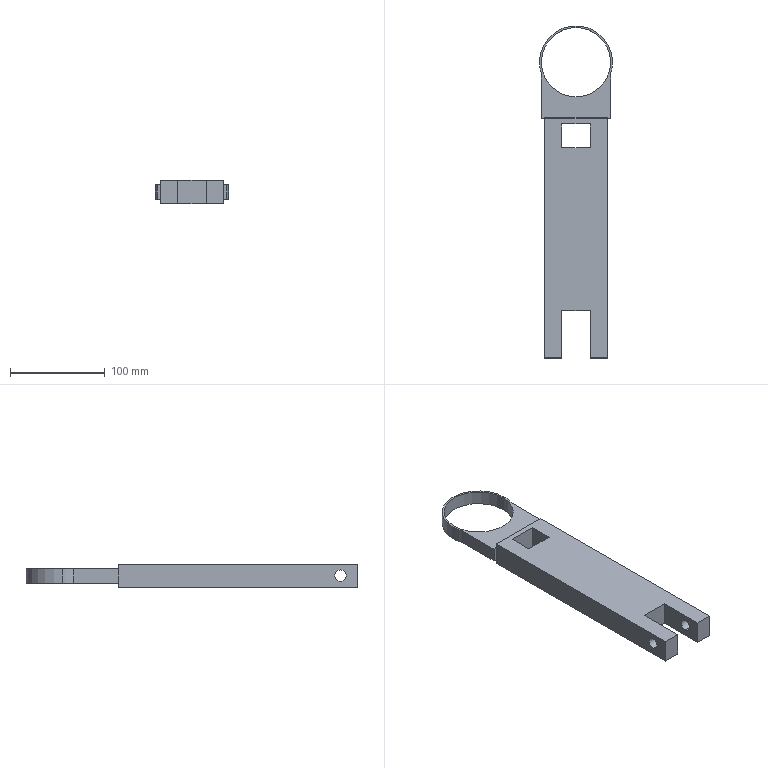Part | SolidWorks | features ICE 3, 3DProfileFeature 1, BossThin 1, Extrusion 1, Fillet 1, HoleWzd 1, MirrorPattern 1 | 1 solid | 32 faces | box 77 x 350 x 25 mm | volume 393296 mm3 | plane 21 | cylinder 11 | commonest cylinder face diameters 12 x4 77 x3 2 x2 73 x2
STEP:
#1=CARTESIAN_POINT('',(-38.5,161.5,-7.5));
#2=VERTEX_POINT('',#1);
#3=CARTESIAN_POINT('',(38.5,161.5,-7.5));
#4=VERTEX_POINT('',#3);
#5=CARTESIAN_POINT('',(0.,161.5,-7.5));
#6=DIRECTION('',(0.,0.,-1.));
#7=DIRECTION('',(-1.,0.,0.));
#8=AXIS2_PLACEMENT_3D('',#5,#6,#7);
#9=CIRCLE('',#8,38.5);
#10=EDGE_CURVE('',#2,#4,#9,.T.);
#11=ORIENTED_EDGE('',*,*,#10,.F.);
#12=CARTESIAN_POINT('',(-38.5,161.5,7.5));
#13=VERTEX_POINT('',#12);
#14=CARTESIAN_POINT('',(-38.5,161.5,-7.5));
#15=DIRECTION('',(0.,0.,1.));
#16=VECTOR('',#15,1000.);
#17=LINE('',#14,#16);
#18=EDGE_CURVE('',#2,#13,#17,.T.);
#19=ORIENTED_EDGE('',*,*,#18,.T.);
#20=CARTESIAN_POINT('',(38.5,161.5,7.5));
#21=VERTEX_POINT('',#20);
#22=CARTESIAN_POINT('',(0.,161.5,7.5));
#23=DIRECTION('',(0.,0.,-1.));
#24=DIRECTION('',(-1.,0.,0.));
#25=AXIS2_PLACEMENT_3D('',#22,#23,#24);
#26=CIRCLE('',#25,38.5);
#27=EDGE_CURVE('',#13,#21,#26,.T.);
#28=ORIENTED_EDGE('',*,*,#27,.T.);
#29=CARTESIAN_POINT('',(38.5,161.5,-7.5));
#30=DIRECTION('',(0.,0.,1.));
#31=VECTOR('',#30,1000.);
#32=LINE('',#29,#31);
#33=EDGE_CURVE('',#4,#21,#32,.T.);
#34=ORIENTED_EDGE('',*,*,#33,.F.);
#35=EDGE_LOOP('',(#11,#19,#28,#34));
#36=FACE_OUTER_BOUND('',#35,.T.);
#37=CARTESIAN_POINT('',(0.,161.5,-7.5));
#38=DIRECTION('',(0.,0.,1.));
#39=DIRECTION('',(1.,0.,0.));
#40=AXIS2_PLACEMENT_3D('',#37,#38,#39);
#41=CYLINDRICAL_SURFACE('',#40,38.5);
#42=ADVANCED_FACE('',(#36),#41,.T.);
#43=CARTESIAN_POINT('',(36.5,149.253,-7.5));
#44=VERTEX_POINT('',#43);
#45=CARTESIAN_POINT('',(0.,161.5,-7.5));
#46=DIRECTION('',(0.,0.,-1.));
#47=DIRECTION('',(-1.,0.,0.));
#48=AXIS2_PLACEMENT_3D('',#45,#46,#47);
#49=CIRCLE('',#48,38.5);
#50=EDGE_CURVE('',#4,#44,#49,.T.);
#51=ORIENTED_EDGE('',*,*,#50,.F.);
#52=ORIENTED_EDGE('',*,*,#33,.T.);
#53=CARTESIAN_POINT('',(36.5,149.253,7.5));
#54=VERTEX_POINT('',#53);
#55=CARTESIAN_POINT('',(0.,161.5,7.5));
#56=DIRECTION('',(0.,0.,-1.));
#57=DIRECTION('',(-1.,0.,0.));
#58=AXIS2_PLACEMENT_3D('',#55,#56,#57);
#59=CIRCLE('',#58,38.5);
#60=EDGE_CURVE('',#21,#54,#59,.T.);
#61=ORIENTED_EDGE('',*,*,#60,.T.);
#62=CARTESIAN_POINT('',(36.5,149.253,-7.5));
#63=DIRECTION('',(0.,0.,-1.));
#64=VECTOR('',#63,1000.);
#65=LINE('',#62,#64);
#66=EDGE_CURVE('',#54,#44,#65,.T.);
#67=ORIENTED_EDGE('',*,*,#66,.T.);
#68=EDGE_LOOP('',(#51,#52,#61,#67));
#69=FACE_OUTER_BOUND('',#68,.T.);
#70=CARTESIAN_POINT('',(0.,161.5,-7.5));
#71=DIRECTION('',(0.,0.,1.));
#72=DIRECTION('',(1.,0.,0.));
#73=AXIS2_PLACEMENT_3D('',#70,#71,#72);
#74=CYLINDRICAL_SURFACE('',#73,38.5);
#75=ADVANCED_FACE('',(#69),#74,.T.);
#76=CARTESIAN_POINT('',(36.5,161.5,-7.5));
#77=VERTEX_POINT('',#76);
#78=CARTESIAN_POINT('',(-36.5,161.5,-7.5));
#79=VERTEX_POINT('',#78);
#80=CARTESIAN_POINT('',(0.,161.5,-7.5));
#81=DIRECTION('',(0.,0.,-1.));
#82=DIRECTION('',(-1.,0.,0.));
#83=AXIS2_PLACEMENT_3D('',#80,#81,#82);
#84=CIRCLE('',#83,36.5);
#85=EDGE_CURVE('',#77,#79,#84,.T.);
#86=ORIENTED_EDGE('',*,*,#85,.T.);
#87=CARTESIAN_POINT('',(-36.5,161.5,7.5));
#88=VERTEX_POINT('',#87);
#89=CARTESIAN_POINT('',(-36.5,161.5,-7.5));
#90=DIRECTION('',(0.,0.,1.));
#91=VECTOR('',#90,1000.);
#92=LINE('',#89,#91);
#93=EDGE_CURVE('',#79,#88,#92,.T.);
#94=ORIENTED_EDGE('',*,*,#93,.T.);
#95=CARTESIAN_POINT('',(36.5,161.5,7.5));
#96=VERTEX_POINT('',#95);
#97=CARTESIAN_POINT('',(0.,161.5,7.5));
#98=DIRECTION('',(0.,0.,-1.));
#99=DIRECTION('',(-1.,0.,0.));
#100=AXIS2_PLACEMENT_3D('',#97,#98,#99);
#101=CIRCLE('',#100,36.5);
#102=EDGE_CURVE('',#96,#88,#101,.T.);
#103=ORIENTED_EDGE('',*,*,#102,.F.);
#104=CARTESIAN_POINT('',(36.5,161.5,-7.5));
#105=DIRECTION('',(0.,0.,1.));
#106=VECTOR('',#105,1000.);
#107=LINE('',#104,#106);
#108=EDGE_CURVE('',#77,#96,#107,.T.);
#109=ORIENTED_EDGE('',*,*,#108,.F.);
#110=EDGE_LOOP('',(#86,#94,#103,#109));
#111=FACE_OUTER_BOUND('',#110,.T.);
#112=CARTESIAN_POINT('',(0.,161.5,-7.5));
#113=DIRECTION('',(0.,0.,1.));
#114=DIRECTION('',(1.,0.,0.));
#115=AXIS2_PLACEMENT_3D('',#112,#113,#114);
#116=CYLINDRICAL_SURFACE('',#115,36.5);
#117=ADVANCED_FACE('',(#111),#116,.F.);
#118=CARTESIAN_POINT('',(-15.,-131.5,-5.548));
#119=VERTEX_POINT('',#118);
#120=CARTESIAN_POINT('',(-15.,-131.5,6.452));
#121=VERTEX_POINT('',#120);
#122=CARTESIAN_POINT('',(-15.,-131.5,0.4516));
#123=DIRECTION('',(-1.,0.,0.));
#124=DIRECTION('',(0.,0.,1.));
#125=AXIS2_PLACEMENT_3D('',#122,#123,#124);
#126=CIRCLE('',#125,6.);
#127=EDGE_CURVE('',#119,#121,#126,.T.);
#128=ORIENTED_EDGE('',*,*,#127,.F.);
#129=CARTESIAN_POINT('',(-33.,-131.5,-5.548));
#130=VERTEX_POINT('',#129);
#131=CARTESIAN_POINT('',(-33.,-131.5,-5.548));
#132=DIRECTION('',(-1.,0.,0.));
#133=VECTOR('',#132,1000.);
#134=LINE('',#131,#133);
#135=EDGE_CURVE('',#119,#130,#134,.T.);
#136=ORIENTED_EDGE('',*,*,#135,.T.);
#137=CARTESIAN_POINT('',(-33.,-131.5,6.452));
#138=VERTEX_POINT('',#137);
#139=CARTESIAN_POINT('',(-33.,-131.5,0.4516));
#140=DIRECTION('',(-1.,0.,0.));
#141=DIRECTION('',(0.,0.,1.));
#142=AXIS2_PLACEMENT_3D('',#139,#140,#141);
#143=CIRCLE('',#142,6.);
#144=EDGE_CURVE('',#130,#138,#143,.T.);
#145=ORIENTED_EDGE('',*,*,#144,.T.);
#146=CARTESIAN_POINT('',(-33.,-131.5,6.452));
#147=DIRECTION('',(-1.,0.,0.));
#148=VECTOR('',#147,1000.);
#149=LINE('',#146,#148);
#150=EDGE_CURVE('',#121,#138,#149,.T.);
#151=ORIENTED_EDGE('',*,*,#150,.F.);
#152=EDGE_LOOP('',(#128,#136,#145,#151));
#153=FACE_OUTER_BOUND('',#152,.T.);
#154=CARTESIAN_POINT('',(-33.,-131.5,0.4516));
#155=DIRECTION('',(-1.,0.,0.));
#156=DIRECTION('',(0.,0.,1.));
#157=AXIS2_PLACEMENT_3D('',#154,#155,#156);
#158=CYLINDRICAL_SURFACE('',#157,6.);
#159=ADVANCED_FACE('',(#153),#158,.F.);
#160=CARTESIAN_POINT('',(15.,-131.5,6.452));
#161=VERTEX_POINT('',#160);
#162=CARTESIAN_POINT('',(15.,-131.5,-5.548));
#163=VERTEX_POINT('',#162);
#164=CARTESIAN_POINT('',(15.,-131.5,0.4516));
#165=DIRECTION('',(1.,0.,0.));
#166=DIRECTION('',(0.,1.,0.));
#167=AXIS2_PLACEMENT_3D('',#164,#165,#166);
#168=CIRCLE('',#167,6.);
#169=EDGE_CURVE('',#161,#163,#168,.T.);
#170=ORIENTED_EDGE('',*,*,#169,.F.);
#171=CARTESIAN_POINT('',(33.,-131.5,6.452));
#172=VERTEX_POINT('',#171);
#173=CARTESIAN_POINT('',(33.,-131.5,6.452));
#174=DIRECTION('',(1.,0.,0.));
#175=VECTOR('',#174,1000.);
#176=LINE('',#173,#175);
#177=EDGE_CURVE('',#161,#172,#176,.T.);
#178=ORIENTED_EDGE('',*,*,#177,.T.);
#179=CARTESIAN_POINT('',(33.,-131.5,-5.548));
#180=VERTEX_POINT('',#179);
#181=CARTESIAN_POINT('',(33.,-131.5,0.4516));
#182=DIRECTION('',(1.,0.,0.));
#183=DIRECTION('',(0.,0.,-1.));
#184=AXIS2_PLACEMENT_3D('',#181,#182,#183);
#185=CIRCLE('',#184,6.);
#186=EDGE_CURVE('',#172,#180,#185,.T.);
#187=ORIENTED_EDGE('',*,*,#186,.T.);
#188=CARTESIAN_POINT('',(33.,-131.5,-5.548));
#189=DIRECTION('',(1.,0.,0.));
#190=VECTOR('',#189,1000.);
#191=LINE('',#188,#190);
#192=EDGE_CURVE('',#163,#180,#191,.T.);
#193=ORIENTED_EDGE('',*,*,#192,.F.);
#194=EDGE_LOOP('',(#170,#178,#187,#193));
#195=FACE_OUTER_BOUND('',#194,.T.);
#196=CARTESIAN_POINT('',(33.,-131.5,0.4516));
#197=DIRECTION('',(1.,0.,0.));
#198=DIRECTION('',(0.,0.,-1.));
#199=AXIS2_PLACEMENT_3D('',#196,#197,#198);
#200=CYLINDRICAL_SURFACE('',#199,6.);
#201=ADVANCED_FACE('',(#195),#200,.F.);
#202=CARTESIAN_POINT('',(-36.5,149.253,7.5));
#203=VERTEX_POINT('',#202);
#204=CARTESIAN_POINT('',(-36.5,102.,7.5));
#205=VERTEX_POINT('',#204);
#206=CARTESIAN_POINT('',(-36.5,0.,7.5));
#207=DIRECTION('',(0.,-1.,0.));
#208=VECTOR('',#207,1000.);
#209=LINE('',#206,#208);
#210=EDGE_CURVE('',#203,#205,#209,.T.);
#211=ORIENTED_EDGE('',*,*,#210,.F.);
#212=CARTESIAN_POINT('',(-36.5,149.253,-7.5));
#213=VERTEX_POINT('',#212);
#214=CARTESIAN_POINT('',(-36.5,149.253,-7.5));
#215=DIRECTION('',(0.,0.,-1.));
#216=VECTOR('',#215,1000.);
#217=LINE('',#214,#216);
#218=EDGE_CURVE('',#203,#213,#217,.T.);
#219=ORIENTED_EDGE('',*,*,#218,.T.);
#220=CARTESIAN_POINT('',(-36.5,102.,-7.5));
#221=VERTEX_POINT('',#220);
#222=CARTESIAN_POINT('',(-36.5,0.,-7.5));
#223=DIRECTION('',(0.,-1.,0.));
#224=VECTOR('',#223,1000.);
#225=LINE('',#222,#224);
#226=EDGE_CURVE('',#213,#221,#225,.T.);
#227=ORIENTED_EDGE('',*,*,#226,.T.);
#228=CARTESIAN_POINT('',(-36.5,102.,-7.5));
#229=DIRECTION('',(0.,0.,1.));
#230=VECTOR('',#229,1000.);
#231=LINE('',#228,#230);
#232=EDGE_CURVE('',#221,#205,#231,.T.);
#233=ORIENTED_EDGE('',*,*,#232,.T.);
#234=EDGE_LOOP('',(#211,#219,#227,#233));
#235=FACE_OUTER_BOUND('',#234,.T.);
#236=CARTESIAN_POINT('',(-36.5,0.,-7.5));
#237=DIRECTION('',(-1.,0.,0.));
#238=DIRECTION('',(0.,-1.,0.));
#239=AXIS2_PLACEMENT_3D('',#236,#237,#238);
#240=PLANE('',#239);
#241=ADVANCED_FACE('',(#235),#240,.T.);
#242=ORIENTED_EDGE('',*,*,#66,.F.);
#243=CARTESIAN_POINT('',(36.5,102.,7.5));
#244=VERTEX_POINT('',#243);
#245=CARTESIAN_POINT('',(36.5,0.,7.5));
#246=DIRECTION('',(0.,-1.,0.));
#247=VECTOR('',#246,1000.);
#248=LINE('',#245,#247);
#249=EDGE_CURVE('',#54,#244,#248,.T.);
#250=ORIENTED_EDGE('',*,*,#249,.T.);
#251=CARTESIAN_POINT('',(36.5,102.,-7.5));
#252=VERTEX_POINT('',#251);
#253=CARTESIAN_POINT('',(36.5,102.,-7.5));
#254=DIRECTION('',(0.,0.,1.));
#255=VECTOR('',#254,1000.);
#256=LINE('',#253,#255);
#257=EDGE_CURVE('',#252,#244,#256,.T.);
#258=ORIENTED_EDGE('',*,*,#257,.F.);
#259=CARTESIAN_POINT('',(36.5,0.,-7.5));
#260=DIRECTION('',(0.,-1.,0.));
#261=VECTOR('',#260,1000.);
#262=LINE('',#259,#261);
#263=EDGE_CURVE('',#44,#252,#262,.T.);
#264=ORIENTED_EDGE('',*,*,#263,.F.);
#265=EDGE_LOOP('',(#242,#250,#258,#264));
#266=FACE_OUTER_BOUND('',#265,.T.);
#267=CARTESIAN_POINT('',(36.5,0.,-7.5));
#268=DIRECTION('',(-1.,0.,0.));
#269=DIRECTION('',(0.,0.,1.));
#270=AXIS2_PLACEMENT_3D('',#267,#268,#269);
#271=PLANE('',#270);
#272=ADVANCED_FACE('',(#266),#271,.F.);
#273=CARTESIAN_POINT('',(-33.,102.,-12.5));
#274=VERTEX_POINT('',#273);
#275=CARTESIAN_POINT('',(-33.,102.,-8.5));
#276=VERTEX_POINT('',#275);
#277=CARTESIAN_POINT('',(-33.,102.,-12.5));
#278=DIRECTION('',(0.,0.,1.));
#279=VECTOR('',#278,1000.);
#280=LINE('',#277,#279);
#281=EDGE_CURVE('',#274,#276,#280,.T.);
#282=ORIENTED_EDGE('',*,*,#281,.T.);
#283=CARTESIAN_POINT('',(33.,102.,-8.5));
#284=VERTEX_POINT('',#283);
#285=CARTESIAN_POINT('',(33.,102.,-8.5));
#286=DIRECTION('',(1.,0.,0.));
#287=VECTOR('',#286,1000.);
#288=LINE('',#285,#287);
#289=EDGE_CURVE('',#276,#284,#288,.T.);
#290=ORIENTED_EDGE('',*,*,#289,.T.);
#291=CARTESIAN_POINT('',(33.,102.,-12.5));
#292=VERTEX_POINT('',#291);
#293=CARTESIAN_POINT('',(33.,102.,12.5));
#294=DIRECTION('',(0.,0.,-1.));
#295=VECTOR('',#294,1000.);
#296=LINE('',#293,#295);
#297=EDGE_CURVE('',#284,#292,#296,.T.);
#298=ORIENTED_EDGE('',*,*,#297,.T.);
#299=CARTESIAN_POINT('',(33.,102.,-12.5));
#300=DIRECTION('',(-1.,0.,0.));
#301=VECTOR('',#300,1000.);
#302=LINE('',#299,#301);
#303=EDGE_CURVE('',#292,#274,#302,.T.);
#304=ORIENTED_EDGE('',*,*,#303,.T.);
#305=EDGE_LOOP('',(#282,#290,#298,#304));
#306=FACE_OUTER_BOUND('',#305,.T.);
#307=CARTESIAN_POINT('',(0.,102.,0.));
#308=DIRECTION('',(0.,1.,0.));
#309=DIRECTION('',(0.,0.,1.));
#310=AXIS2_PLACEMENT_3D('',#307,#308,#309);
#311=PLANE('',#310);
#312=ADVANCED_FACE('',(#306),#311,.T.);
#313=CARTESIAN_POINT('',(33.,-150.,12.5));
#314=VERTEX_POINT('',#313);
#315=CARTESIAN_POINT('',(33.,102.,12.5));
#316=VERTEX_POINT('',#315);
#317=CARTESIAN_POINT('',(33.,-150.,12.5));
#318=DIRECTION('',(0.,1.,0.));
#319=VECTOR('',#318,1000.);
#320=LINE('',#317,#319);
#321=EDGE_CURVE('',#314,#316,#320,.T.);
#322=ORIENTED_EDGE('',*,*,#321,.T.);
#323=CARTESIAN_POINT('',(-33.,102.,12.5));
#324=VERTEX_POINT('',#323);
#325=CARTESIAN_POINT('',(-33.,102.,12.5));
#326=DIRECTION('',(1.,0.,0.));
#327=VECTOR('',#326,1000.);
#328=LINE('',#325,#327);
#329=EDGE_CURVE('',#324,#316,#328,.T.);
#330=ORIENTED_EDGE('',*,*,#329,.F.);
#331=CARTESIAN_POINT('',(-33.,-150.,12.5));
#332=VERTEX_POINT('',#331);
#333=CARTESIAN_POINT('',(-33.,-150.,12.5));
#334=DIRECTION('',(0.,-1.,0.));
#335=VECTOR('',#334,1000.);
#336=LINE('',#333,#335);
#337=EDGE_CURVE('',#324,#332,#336,.T.);
#338=ORIENTED_EDGE('',*,*,#337,.T.);
#339=CARTESIAN_POINT('',(-15.,-150.,12.5));
#340=VERTEX_POINT('',#339);
#341=CARTESIAN_POINT('',(-33.,-150.,12.5));
#342=DIRECTION('',(1.,0.,0.));
#343=VECTOR('',#342,1000.);
#344=LINE('',#341,#343);
#345=EDGE_CURVE('',#332,#340,#344,.T.);
#346=ORIENTED_EDGE('',*,*,#345,.T.);
#347=CARTESIAN_POINT('',(-15.,-100.,12.5));
#348=VERTEX_POINT('',#347);
#349=CARTESIAN_POINT('',(-15.,-100.,12.5));
#350=DIRECTION('',(0.,1.,0.));
#351=VECTOR('',#350,1000.);
#352=LINE('',#349,#351);
#353=EDGE_CURVE('',#340,#348,#352,.T.);
#354=ORIENTED_EDGE('',*,*,#353,.T.);
#355=CARTESIAN_POINT('',(15.,-100.,12.5));
#356=VERTEX_POINT('',#355);
#357=CARTESIAN_POINT('',(0.,-100.,12.5));
#358=DIRECTION('',(1.,0.,0.));
#359=VECTOR('',#358,1000.);
#360=LINE('',#357,#359);
#361=EDGE_CURVE('',#348,#356,#360,.T.);
#362=ORIENTED_EDGE('',*,*,#361,.T.);
#363=CARTESIAN_POINT('',(15.,-150.,12.5));
#364=VERTEX_POINT('',#363);
#365=CARTESIAN_POINT('',(15.,-100.,12.5));
#366=DIRECTION('',(0.,-1.,0.));
#367=VECTOR('',#366,1000.);
#368=LINE('',#365,#367);
#369=EDGE_CURVE('',#356,#364,#368,.T.);
#370=ORIENTED_EDGE('',*,*,#369,.T.);
#371=CARTESIAN_POINT('',(15.,-150.,12.5));
#372=DIRECTION('',(1.,0.,0.));
#373=VECTOR('',#372,1000.);
#374=LINE('',#371,#373);
#375=EDGE_CURVE('',#364,#314,#374,.T.);
#376=ORIENTED_EDGE('',*,*,#375,.T.);
#377=EDGE_LOOP('',(#322,#330,#338,#346,#354,#362,#370,#376));
#378=FACE_OUTER_BOUND('',#377,.T.);
#379=CARTESIAN_POINT('',(15.,96.565,12.5));
#380=VERTEX_POINT('',#379);
#381=CARTESIAN_POINT('',(-15.,96.565,12.5));
#382=VERTEX_POINT('',#381);
#383=CARTESIAN_POINT('',(15.,96.565,12.5));
#384=DIRECTION('',(-1.,0.,0.));
#385=VECTOR('',#384,1000.);
#386=LINE('',#383,#385);
#387=EDGE_CURVE('',#380,#382,#386,.T.);
#388=ORIENTED_EDGE('',*,*,#387,.F.);
#389=CARTESIAN_POINT('',(15.,71.565,12.5));
#390=VERTEX_POINT('',#389);
#391=CARTESIAN_POINT('',(15.,71.565,12.5));
#392=DIRECTION('',(0.,1.,0.));
#393=VECTOR('',#392,1000.);
#394=LINE('',#391,#393);
#395=EDGE_CURVE('',#390,#380,#394,.T.);
#396=ORIENTED_EDGE('',*,*,#395,.F.);
#397=CARTESIAN_POINT('',(-15.,71.565,12.5));
#398=VERTEX_POINT('',#397);
#399=CARTESIAN_POINT('',(15.,71.565,12.5));
#400=DIRECTION('',(-1.,0.,0.));
#401=VECTOR('',#400,1000.);
#402=LINE('',#399,#401);
#403=EDGE_CURVE('',#390,#398,#402,.T.);
#404=ORIENTED_EDGE('',*,*,#403,.T.);
#405=CARTESIAN_POINT('',(-15.,71.565,12.5));
#406=DIRECTION('',(0.,1.,0.));
#407=VECTOR('',#406,1000.);
#408=LINE('',#405,#407);
#409=EDGE_CURVE('',#398,#382,#408,.T.);
#410=ORIENTED_EDGE('',*,*,#409,.T.);
#411=EDGE_LOOP('',(#388,#396,#404,#410));
#412=FACE_BOUND('',#411,.T.);
#413=CARTESIAN_POINT('',(0.,0.,12.5));
#414=DIRECTION('',(0.,0.,1.));
#415=DIRECTION('',(1.,0.,0.));
#416=AXIS2_PLACEMENT_3D('',#413,#414,#415);
#417=PLANE('',#416);
#418=ADVANCED_FACE('',(#378,#412),#417,.T.);
#419=CARTESIAN_POINT('',(-33.,-150.,-12.5));
#420=VERTEX_POINT('',#419);
#421=CARTESIAN_POINT('',(-33.,-150.,-12.5));
#422=DIRECTION('',(0.,-1.,0.));
#423=VECTOR('',#422,1000.);
#424=LINE('',#421,#423);
#425=EDGE_CURVE('',#274,#420,#424,.T.);
#426=ORIENTED_EDGE('',*,*,#425,.F.);
#427=ORIENTED_EDGE('',*,*,#303,.F.);
#428=CARTESIAN_POINT('',(33.,-150.,-12.5));
#429=VERTEX_POINT('',#428);
#430=CARTESIAN_POINT('',(33.,-150.,-12.5));
#431=DIRECTION('',(0.,1.,0.));
#432=VECTOR('',#431,1000.);
#433=LINE('',#430,#432);
#434=EDGE_CURVE('',#429,#292,#433,.T.);
#435=ORIENTED_EDGE('',*,*,#434,.F.);
#436=CARTESIAN_POINT('',(15.,-150.,-12.5));
#437=VERTEX_POINT('',#436);
#438=CARTESIAN_POINT('',(15.,-150.,-12.5));
#439=DIRECTION('',(1.,0.,0.));
#440=VECTOR('',#439,1000.);
#441=LINE('',#438,#440);
#442=EDGE_CURVE('',#437,#429,#441,.T.);
#443=ORIENTED_EDGE('',*,*,#442,.F.);
#444=CARTESIAN_POINT('',(15.,-100.,-12.5));
#445=VERTEX_POINT('',#444);
#446=CARTESIAN_POINT('',(15.,-100.,-12.5));
#447=DIRECTION('',(0.,-1.,0.));
#448=VECTOR('',#447,1000.);
#449=LINE('',#446,#448);
#450=EDGE_CURVE('',#445,#437,#449,.T.);
#451=ORIENTED_EDGE('',*,*,#450,.F.);
#452=CARTESIAN_POINT('',(-15.,-100.,-12.5));
#453=VERTEX_POINT('',#452);
#454=CARTESIAN_POINT('',(0.,-100.,-12.5));
#455=DIRECTION('',(1.,0.,0.));
#456=VECTOR('',#455,1000.);
#457=LINE('',#454,#456);
#458=EDGE_CURVE('',#453,#445,#457,.T.);
#459=ORIENTED_EDGE('',*,*,#458,.F.);
#460=CARTESIAN_POINT('',(-15.,-150.,-12.5));
#461=VERTEX_POINT('',#460);
#462=CARTESIAN_POINT('',(-15.,-100.,-12.5));
#463=DIRECTION('',(0.,1.,0.));
#464=VECTOR('',#463,1000.);
#465=LINE('',#462,#464);
#466=EDGE_CURVE('',#461,#453,#465,.T.);
#467=ORIENTED_EDGE('',*,*,#466,.F.);
#468=CARTESIAN_POINT('',(-33.,-150.,-12.5));
#469=DIRECTION('',(1.,0.,0.));
#470=VECTOR('',#469,1000.);
#471=LINE('',#468,#470);
#472=EDGE_CURVE('',#420,#461,#471,.T.);
#473=ORIENTED_EDGE('',*,*,#472,.F.);
#474=EDGE_LOOP('',(#426,#427,#435,#443,#451,#459,#467,#473));
#475=FACE_OUTER_BOUND('',#474,.T.);
#476=CARTESIAN_POINT('',(15.,96.565,-12.5));
#477=VERTEX_POINT('',#476);
#478=CARTESIAN_POINT('',(15.,71.565,-12.5));
#479=VERTEX_POINT('',#478);
#480=CARTESIAN_POINT('',(15.,0.,-12.5));
#481=DIRECTION('',(0.,-1.,0.));
#482=VECTOR('',#481,1000.);
#483=LINE('',#480,#482);
#484=EDGE_CURVE('',#477,#479,#483,.T.);
#485=ORIENTED_EDGE('',*,*,#484,.F.);
#486=CARTESIAN_POINT('',(-15.,96.565,-12.5));
#487=VERTEX_POINT('',#486);
#488=CARTESIAN_POINT('',(0.,96.565,-12.5));
#489=DIRECTION('',(1.,0.,0.));
#490=VECTOR('',#489,1000.);
#491=LINE('',#488,#490);
#492=EDGE_CURVE('',#487,#477,#491,.T.);
#493=ORIENTED_EDGE('',*,*,#492,.F.);
#494=CARTESIAN_POINT('',(-15.,71.565,-12.5));
#495=VERTEX_POINT('',#494);
#496=CARTESIAN_POINT('',(-15.,0.,-12.5));
#497=DIRECTION('',(0.,-1.,0.));
#498=VECTOR('',#497,1000.);
#499=LINE('',#496,#498);
#500=EDGE_CURVE('',#487,#495,#499,.T.);
#501=ORIENTED_EDGE('',*,*,#500,.T.);
#502=CARTESIAN_POINT('',(0.,71.565,-12.5));
#503=DIRECTION('',(1.,0.,0.));
#504=VECTOR('',#503,1000.);
#505=LINE('',#502,#504);
#506=EDGE_CURVE('',#495,#479,#505,.T.);
#507=ORIENTED_EDGE('',*,*,#506,.T.);
#508=EDGE_LOOP('',(#485,#493,#501,#507));
#509=FACE_BOUND('',#508,.T.);
#510=CARTESIAN_POINT('',(0.,0.,-12.5));
#511=DIRECTION('',(0.,0.,1.));
#512=DIRECTION('',(1.,0.,0.));
#513=AXIS2_PLACEMENT_3D('',#510,#511,#512);
#514=PLANE('',#513);
#515=ADVANCED_FACE('',(#475,#509),#514,.F.);
#516=ORIENTED_EDGE('',*,*,#425,.T.);
#517=CARTESIAN_POINT('',(-33.,-150.,12.5));
#518=DIRECTION('',(0.,0.,-1.));
#519=VECTOR('',#518,1000.);
#520=LINE('',#517,#519);
#521=EDGE_CURVE('',#332,#420,#520,.T.);
#522=ORIENTED_EDGE('',*,*,#521,.F.);
#523=ORIENTED_EDGE('',*,*,#337,.F.);
#524=CARTESIAN_POINT('',(-33.,102.,8.5));
#525=VERTEX_POINT('',#524);
#526=CARTESIAN_POINT('',(-33.,102.,-12.5));
#527=DIRECTION('',(0.,0.,1.));
#528=VECTOR('',#527,1000.);
#529=LINE('',#526,#528);
#530=EDGE_CURVE('',#525,#324,#529,.T.);
#531=ORIENTED_EDGE('',*,*,#530,.F.);
#532=CARTESIAN_POINT('',(-33.,103.,7.5));
#533=VERTEX_POINT('',#532);
#534=CARTESIAN_POINT('',(-33.,103.,8.5));
#535=DIRECTION('',(1.,0.,0.));
#536=DIRECTION('',(0.,0.,-1.));
#537=AXIS2_PLACEMENT_3D('',#534,#535,#536);
#538=CIRCLE('',#537,1.);
#539=EDGE_CURVE('',#525,#533,#538,.T.);
#540=ORIENTED_EDGE('',*,*,#539,.T.);
#541=CARTESIAN_POINT('',(-33.,102.,7.5));
#542=VERTEX_POINT('',#541);
#543=CARTESIAN_POINT('',(-33.,-150.,7.5));
#544=DIRECTION('',(0.,1.,0.));
#545=VECTOR('',#544,1000.);
#546=LINE('',#543,#545);
#547=EDGE_CURVE('',#542,#533,#546,.T.);
#548=ORIENTED_EDGE('',*,*,#547,.F.);
#549=CARTESIAN_POINT('',(-33.,102.,-7.5));
#550=VERTEX_POINT('',#549);
#551=CARTESIAN_POINT('',(-33.,102.,-12.5));
#552=DIRECTION('',(0.,0.,1.));
#553=VECTOR('',#552,1000.);
#554=LINE('',#551,#553);
#555=EDGE_CURVE('',#550,#542,#554,.T.);
#556=ORIENTED_EDGE('',*,*,#555,.F.);
#557=CARTESIAN_POINT('',(-33.,103.,-7.5));
#558=VERTEX_POINT('',#557);
#559=CARTESIAN_POINT('',(-33.,0.,-7.5));
#560=DIRECTION('',(0.,-1.,0.));
#561=VECTOR('',#560,1000.);
#562=LINE('',#559,#561);
#563=EDGE_CURVE('',#558,#550,#562,.T.);
#564=ORIENTED_EDGE('',*,*,#563,.F.);
#565=CARTESIAN_POINT('',(-33.,103.,-8.5));
#566=DIRECTION('',(1.,0.,0.));
#567=DIRECTION('',(0.,0.,-1.));
#568=AXIS2_PLACEMENT_3D('',#565,#566,#567);
#569=CIRCLE('',#568,1.);
#570=EDGE_CURVE('',#558,#276,#569,.T.);
#571=ORIENTED_EDGE('',*,*,#570,.T.);
#572=ORIENTED_EDGE('',*,*,#281,.F.);
#573=EDGE_LOOP('',(#516,#522,#523,#531,#540,#548,#556,#564,#571,#572));
#574=FACE_OUTER_BOUND('',#573,.T.);
#575=CARTESIAN_POINT('',(-33.,-131.5,0.4516));
#576=DIRECTION('',(-1.,0.,0.));
#577=DIRECTION('',(0.,0.,1.));
#578=AXIS2_PLACEMENT_3D('',#575,#576,#577);
#579=CIRCLE('',#578,6.);
#580=EDGE_CURVE('',#138,#130,#579,.T.);
#581=ORIENTED_EDGE('',*,*,#580,.F.);
#582=ORIENTED_EDGE('',*,*,#144,.F.);
#583=EDGE_LOOP('',(#581,#582));
#584=FACE_BOUND('',#583,.T.);
#585=CARTESIAN_POINT('',(-33.,-150.,12.5));
#586=DIRECTION('',(1.,0.,0.));
#587=DIRECTION('',(0.,0.,-1.));
#588=AXIS2_PLACEMENT_3D('',#585,#586,#587);
#589=PLANE('',#588);
#590=ADVANCED_FACE('',(#574,#584),#589,.F.);
#591=ORIENTED_EDGE('',*,*,#434,.T.);
#592=ORIENTED_EDGE('',*,*,#297,.F.);
#593=CARTESIAN_POINT('',(33.,103.,-7.5));
#594=VERTEX_POINT('',#593);
#595=CARTESIAN_POINT('',(33.,103.,-8.5));
#596=DIRECTION('',(-1.,0.,0.));
#597=DIRECTION('',(0.,-1.,0.));
#598=AXIS2_PLACEMENT_3D('',#595,#596,#597);
#599=CIRCLE('',#598,1.);
#600=EDGE_CURVE('',#284,#594,#599,.T.);
#601=ORIENTED_EDGE('',*,*,#600,.T.);
#602=CARTESIAN_POINT('',(33.,102.,-7.5));
#603=VERTEX_POINT('',#602);
#604=CARTESIAN_POINT('',(33.,0.,-7.5));
#605=DIRECTION('',(0.,1.,0.));
#606=VECTOR('',#605,1000.);
#607=LINE('',#604,#606);
#608=EDGE_CURVE('',#603,#594,#607,.T.);
#609=ORIENTED_EDGE('',*,*,#608,.F.);
#610=CARTESIAN_POINT('',(33.,102.,7.5));
#611=VERTEX_POINT('',#610);
#612=CARTESIAN_POINT('',(33.,102.,12.5));
#613=DIRECTION('',(0.,0.,-1.));
#614=VECTOR('',#613,1000.);
#615=LINE('',#612,#614);
#616=EDGE_CURVE('',#611,#603,#615,.T.);
#617=ORIENTED_EDGE('',*,*,#616,.F.);
#618=CARTESIAN_POINT('',(33.,103.,7.5));
#619=VERTEX_POINT('',#618);
#620=CARTESIAN_POINT('',(33.,-150.,7.5));
#621=DIRECTION('',(0.,-1.,0.));
#622=VECTOR('',#621,1000.);
#623=LINE('',#620,#622);
#624=EDGE_CURVE('',#619,#611,#623,.T.);
#625=ORIENTED_EDGE('',*,*,#624,.F.);
#626=CARTESIAN_POINT('',(33.,102.,8.5));
#627=VERTEX_POINT('',#626);
#628=CARTESIAN_POINT('',(33.,103.,8.5));
#629=DIRECTION('',(-1.,0.,0.));
#630=DIRECTION('',(0.,-1.,0.));
#631=AXIS2_PLACEMENT_3D('',#628,#629,#630);
#632=CIRCLE('',#631,1.);
#633=EDGE_CURVE('',#619,#627,#632,.T.);
#634=ORIENTED_EDGE('',*,*,#633,.T.);
#635=CARTESIAN_POINT('',(33.,102.,12.5));
#636=DIRECTION('',(0.,0.,-1.));
#637=VECTOR('',#636,1000.);
#638=LINE('',#635,#637);
#639=EDGE_CURVE('',#316,#627,#638,.T.);
#640=ORIENTED_EDGE('',*,*,#639,.F.);
#641=ORIENTED_EDGE('',*,*,#321,.F.);
#642=CARTESIAN_POINT('',(33.,-150.,12.5));
#643=DIRECTION('',(0.,0.,-1.));
#644=VECTOR('',#643,1000.);
#645=LINE('',#642,#644);
#646=EDGE_CURVE('',#314,#429,#645,.T.);
#647=ORIENTED_EDGE('',*,*,#646,.T.);
#648=EDGE_LOOP('',(#591,#592,#601,#609,#617,#625,#634,#640,#641,#647));
#649=FACE_OUTER_BOUND('',#648,.T.);
#650=CARTESIAN_POINT('',(33.,-131.5,0.4516));
#651=DIRECTION('',(1.,0.,0.));
#652=DIRECTION('',(0.,0.,-1.));
#653=AXIS2_PLACEMENT_3D('',#650,#651,#652);
#654=CIRCLE('',#653,6.);
#655=EDGE_CURVE('',#180,#172,#654,.T.);
#656=ORIENTED_EDGE('',*,*,#655,.F.);
#657=ORIENTED_EDGE('',*,*,#186,.F.);
#658=EDGE_LOOP('',(#656,#657));
#659=FACE_BOUND('',#658,.T.);
#660=CARTESIAN_POINT('',(33.,-150.,12.5));
#661=DIRECTION('',(-1.,0.,0.));
#662=DIRECTION('',(0.,-1.,0.));
#663=AXIS2_PLACEMENT_3D('',#660,#661,#662);
#664=PLANE('',#663);
#665=ADVANCED_FACE('',(#649,#659),#664,.F.);
#666=ORIENTED_EDGE('',*,*,#472,.T.);
#667=CARTESIAN_POINT('',(-15.,-150.,12.5));
#668=DIRECTION('',(0.,0.,-1.));
#669=VECTOR('',#668,1000.);
#670=LINE('',#667,#669);
#671=EDGE_CURVE('',#340,#461,#670,.T.);
#672=ORIENTED_EDGE('',*,*,#671,.F.);
#673=ORIENTED_EDGE('',*,*,#345,.F.);
#674=ORIENTED_EDGE('',*,*,#521,.T.);
#675=EDGE_LOOP('',(#666,#672,#673,#674));
#676=FACE_OUTER_BOUND('',#675,.T.);
#677=CARTESIAN_POINT('',(-33.,-150.,12.5));
#678=DIRECTION('',(0.,1.,0.));
#679=DIRECTION('',(0.,0.,1.));
#680=AXIS2_PLACEMENT_3D('',#677,#678,#679);
#681=PLANE('',#680);
#682=ADVANCED_FACE('',(#676),#681,.F.);
#683=CARTESIAN_POINT('',(-15.,-131.5,0.4516));
#684=DIRECTION('',(-1.,0.,0.));
#685=DIRECTION('',(0.,0.,1.));
#686=AXIS2_PLACEMENT_3D('',#683,#684,#685);
#687=CIRCLE('',#686,6.);
#688=EDGE_CURVE('',#121,#119,#687,.T.);
#689=ORIENTED_EDGE('',*,*,#688,.T.);
#690=ORIENTED_EDGE('',*,*,#127,.T.);
#691=EDGE_LOOP('',(#689,#690));
#692=FACE_BOUND('',#691,.T.);
#693=ORIENTED_EDGE('',*,*,#466,.T.);
#694=CARTESIAN_POINT('',(-15.,-100.,12.5));
#695=DIRECTION('',(0.,0.,-1.));
#696=VECTOR('',#695,1000.);
#697=LINE('',#694,#696);
#698=EDGE_CURVE('',#348,#453,#697,.T.);
#699=ORIENTED_EDGE('',*,*,#698,.F.);
#700=ORIENTED_EDGE('',*,*,#353,.F.);
#701=ORIENTED_EDGE('',*,*,#671,.T.);
#702=EDGE_LOOP('',(#693,#699,#700,#701));
#703=FACE_OUTER_BOUND('',#702,.T.);
#704=CARTESIAN_POINT('',(-15.,-100.,12.5));
#705=DIRECTION('',(-1.,0.,0.));
#706=DIRECTION('',(0.,0.,1.));
#707=AXIS2_PLACEMENT_3D('',#704,#705,#706);
#708=PLANE('',#707);
#709=ADVANCED_FACE('',(#692,#703),#708,.F.);
#710=ORIENTED_EDGE('',*,*,#458,.T.);
#711=CARTESIAN_POINT('',(15.,-100.,12.5));
#712=DIRECTION('',(0.,0.,-1.));
#713=VECTOR('',#712,1000.);
#714=LINE('',#711,#713);
#715=EDGE_CURVE('',#356,#445,#714,.T.);
#716=ORIENTED_EDGE('',*,*,#715,.F.);
#717=ORIENTED_EDGE('',*,*,#361,.F.);
#718=ORIENTED_EDGE('',*,*,#698,.T.);
#719=EDGE_LOOP('',(#710,#716,#717,#718));
#720=FACE_OUTER_BOUND('',#719,.T.);
#721=CARTESIAN_POINT('',(0.,-100.,12.5));
#722=DIRECTION('',(0.,1.,0.));
#723=DIRECTION('',(0.,0.,1.));
#724=AXIS2_PLACEMENT_3D('',#721,#722,#723);
#725=PLANE('',#724);
#726=ADVANCED_FACE('',(#720),#725,.F.);
#727=CARTESIAN_POINT('',(15.,-131.5,0.4516));
#728=DIRECTION('',(1.,0.,0.));
#729=DIRECTION('',(0.,1.,0.));
#730=AXIS2_PLACEMENT_3D('',#727,#728,#729);
#731=CIRCLE('',#730,6.);
#732=EDGE_CURVE('',#163,#161,#731,.T.);
#733=ORIENTED_EDGE('',*,*,#732,.T.);
#734=ORIENTED_EDGE('',*,*,#169,.T.);
#735=EDGE_LOOP('',(#733,#734));
#736=FACE_BOUND('',#735,.T.);
#737=ORIENTED_EDGE('',*,*,#450,.T.);
#738=CARTESIAN_POINT('',(15.,-150.,12.5));
#739=DIRECTION('',(0.,0.,-1.));
#740=VECTOR('',#739,1000.);
#741=LINE('',#738,#740);
#742=EDGE_CURVE('',#364,#437,#741,.T.);
#743=ORIENTED_EDGE('',*,*,#742,.F.);
#744=ORIENTED_EDGE('',*,*,#369,.F.);
#745=ORIENTED_EDGE('',*,*,#715,.T.);
#746=EDGE_LOOP('',(#737,#743,#744,#745));
#747=FACE_OUTER_BOUND('',#746,.T.);
#748=CARTESIAN_POINT('',(15.,-100.,12.5));
#749=DIRECTION('',(1.,0.,0.));
#750=DIRECTION('',(0.,1.,0.));
#751=AXIS2_PLACEMENT_3D('',#748,#749,#750);
#752=PLANE('',#751);
#753=ADVANCED_FACE('',(#736,#747),#752,.F.);
#754=ORIENTED_EDGE('',*,*,#442,.T.);
#755=ORIENTED_EDGE('',*,*,#646,.F.);
#756=ORIENTED_EDGE('',*,*,#375,.F.);
#757=ORIENTED_EDGE('',*,*,#742,.T.);
#758=EDGE_LOOP('',(#754,#755,#756,#757));
#759=FACE_OUTER_BOUND('',#758,.T.);
#760=CARTESIAN_POINT('',(15.,-150.,12.5));
#761=DIRECTION('',(0.,1.,0.));
#762=DIRECTION('',(0.,0.,1.));
#763=AXIS2_PLACEMENT_3D('',#760,#761,#762);
#764=PLANE('',#763);
#765=ADVANCED_FACE('',(#759),#764,.F.);
#766=ORIENTED_EDGE('',*,*,#177,.F.);
#767=ORIENTED_EDGE('',*,*,#732,.F.);
#768=ORIENTED_EDGE('',*,*,#192,.T.);
#769=ORIENTED_EDGE('',*,*,#655,.T.);
#770=EDGE_LOOP('',(#766,#767,#768,#769));
#771=FACE_OUTER_BOUND('',#770,.T.);
#772=CARTESIAN_POINT('',(33.,-131.5,0.4516));
#773=DIRECTION('',(1.,0.,0.));
#774=DIRECTION('',(0.,0.,-1.));
#775=AXIS2_PLACEMENT_3D('',#772,#773,#774);
#776=CYLINDRICAL_SURFACE('',#775,6.);
#777=ADVANCED_FACE('',(#771),#776,.F.);
#778=ORIENTED_EDGE('',*,*,#135,.F.);
#779=ORIENTED_EDGE('',*,*,#688,.F.);
#780=ORIENTED_EDGE('',*,*,#150,.T.);
#781=ORIENTED_EDGE('',*,*,#580,.T.);
#782=EDGE_LOOP('',(#778,#779,#780,#781));
#783=FACE_OUTER_BOUND('',#782,.T.);
#784=CARTESIAN_POINT('',(-33.,-131.5,0.4516));
#785=DIRECTION('',(-1.,0.,0.));
#786=DIRECTION('',(0.,0.,1.));
#787=AXIS2_PLACEMENT_3D('',#784,#785,#786);
#788=CYLINDRICAL_SURFACE('',#787,6.);
#789=ADVANCED_FACE('',(#783),#788,.F.);
#790=ORIENTED_EDGE('',*,*,#639,.T.);
#791=CARTESIAN_POINT('',(0.,102.,8.5));
#792=DIRECTION('',(-1.,0.,0.));
#793=VECTOR('',#792,1000.);
#794=LINE('',#791,#793);
#795=EDGE_CURVE('',#627,#525,#794,.T.);
#796=ORIENTED_EDGE('',*,*,#795,.T.);
#797=ORIENTED_EDGE('',*,*,#530,.T.);
#798=ORIENTED_EDGE('',*,*,#329,.T.);
#799=EDGE_LOOP('',(#790,#796,#797,#798));
#800=FACE_OUTER_BOUND('',#799,.T.);
#801=CARTESIAN_POINT('',(0.,102.,0.));
#802=DIRECTION('',(0.,1.,0.));
#803=DIRECTION('',(0.,0.,1.));
#804=AXIS2_PLACEMENT_3D('',#801,#802,#803);
#805=PLANE('',#804);
#806=ADVANCED_FACE('',(#800),#805,.T.);
#807=ORIENTED_EDGE('',*,*,#484,.T.);
#808=CARTESIAN_POINT('',(15.,71.565,12.5));
#809=DIRECTION('',(0.,0.,-1.));
#810=VECTOR('',#809,1000.);
#811=LINE('',#808,#810);
#812=EDGE_CURVE('',#390,#479,#811,.T.);
#813=ORIENTED_EDGE('',*,*,#812,.F.);
#814=ORIENTED_EDGE('',*,*,#395,.T.);
#815=CARTESIAN_POINT('',(15.,96.565,12.5));
#816=DIRECTION('',(0.,0.,-1.));
#817=VECTOR('',#816,1000.);
#818=LINE('',#815,#817);
#819=EDGE_CURVE('',#380,#477,#818,.T.);
#820=ORIENTED_EDGE('',*,*,#819,.T.);
#821=EDGE_LOOP('',(#807,#813,#814,#820));
#822=FACE_OUTER_BOUND('',#821,.T.);
#823=CARTESIAN_POINT('',(15.,71.565,12.5));
#824=DIRECTION('',(-1.,0.,0.));
#825=DIRECTION('',(0.,0.,1.));
#826=AXIS2_PLACEMENT_3D('',#823,#824,#825);
#827=PLANE('',#826);
#828=ADVANCED_FACE('',(#822),#827,.T.);
#829=ORIENTED_EDGE('',*,*,#492,.T.);
#830=ORIENTED_EDGE('',*,*,#819,.F.);
#831=ORIENTED_EDGE('',*,*,#387,.T.);
#832=CARTESIAN_POINT('',(-15.,96.565,12.5));
#833=DIRECTION('',(0.,0.,-1.));
#834=VECTOR('',#833,1000.);
#835=LINE('',#832,#834);
#836=EDGE_CURVE('',#382,#487,#835,.T.);
#837=ORIENTED_EDGE('',*,*,#836,.T.);
#838=EDGE_LOOP('',(#829,#830,#831,#837));
#839=FACE_OUTER_BOUND('',#838,.T.);
#840=CARTESIAN_POINT('',(15.,96.565,12.5));
#841=DIRECTION('',(0.,-1.,0.));
#842=DIRECTION('',(0.,0.,-1.));
#843=AXIS2_PLACEMENT_3D('',#840,#841,#842);
#844=PLANE('',#843);
#845=ADVANCED_FACE('',(#839),#844,.T.);
#846=ORIENTED_EDGE('',*,*,#836,.F.);
#847=ORIENTED_EDGE('',*,*,#409,.F.);
#848=CARTESIAN_POINT('',(-15.,71.565,12.5));
#849=DIRECTION('',(0.,0.,-1.));
#850=VECTOR('',#849,1000.);
#851=LINE('',#848,#850);
#852=EDGE_CURVE('',#398,#495,#851,.T.);
#853=ORIENTED_EDGE('',*,*,#852,.T.);
#854=ORIENTED_EDGE('',*,*,#500,.F.);
#855=EDGE_LOOP('',(#846,#847,#853,#854));
#856=FACE_OUTER_BOUND('',#855,.T.);
#857=CARTESIAN_POINT('',(-15.,71.565,12.5));
#858=DIRECTION('',(-1.,0.,0.));
#859=DIRECTION('',(0.,0.,1.));
#860=AXIS2_PLACEMENT_3D('',#857,#858,#859);
#861=PLANE('',#860);
#862=ADVANCED_FACE('',(#856),#861,.F.);
#863=ORIENTED_EDGE('',*,*,#852,.F.);
#864=ORIENTED_EDGE('',*,*,#403,.F.);
#865=ORIENTED_EDGE('',*,*,#812,.T.);
#866=ORIENTED_EDGE('',*,*,#506,.F.);
#867=EDGE_LOOP('',(#863,#864,#865,#866));
#868=FACE_OUTER_BOUND('',#867,.T.);
#869=CARTESIAN_POINT('',(15.,71.565,12.5));
#870=DIRECTION('',(0.,-1.,0.));
#871=DIRECTION('',(0.,0.,-1.));
#872=AXIS2_PLACEMENT_3D('',#869,#870,#871);
#873=PLANE('',#872);
#874=ADVANCED_FACE('',(#868),#873,.F.);
#875=CARTESIAN_POINT('',(0.,102.,7.5));
#876=DIRECTION('',(1.,0.,0.));
#877=VECTOR('',#876,1000.);
#878=LINE('',#875,#877);
#879=EDGE_CURVE('',#611,#244,#878,.T.);
#880=ORIENTED_EDGE('',*,*,#879,.F.);
#881=ORIENTED_EDGE('',*,*,#616,.T.);
#882=CARTESIAN_POINT('',(0.,102.,-7.5));
#883=DIRECTION('',(1.,0.,0.));
#884=VECTOR('',#883,1000.);
#885=LINE('',#882,#884);
#886=EDGE_CURVE('',#603,#252,#885,.T.);
#887=ORIENTED_EDGE('',*,*,#886,.T.);
#888=ORIENTED_EDGE('',*,*,#257,.T.);
#889=EDGE_LOOP('',(#880,#881,#887,#888));
#890=FACE_OUTER_BOUND('',#889,.T.);
#891=CARTESIAN_POINT('',(0.,102.,-7.5));
#892=DIRECTION('',(0.,-1.,0.));
#893=DIRECTION('',(0.,0.,-1.));
#894=AXIS2_PLACEMENT_3D('',#891,#892,#893);
#895=PLANE('',#894);
#896=ADVANCED_FACE('',(#890),#895,.T.);
#897=CARTESIAN_POINT('',(0.,102.,-7.5));
#898=DIRECTION('',(1.,0.,0.));
#899=VECTOR('',#898,1000.);
#900=LINE('',#897,#899);
#901=EDGE_CURVE('',#221,#550,#900,.T.);
#902=ORIENTED_EDGE('',*,*,#901,.T.);
#903=ORIENTED_EDGE('',*,*,#555,.T.);
#904=CARTESIAN_POINT('',(0.,102.,7.5));
#905=DIRECTION('',(1.,0.,0.));
#906=VECTOR('',#905,1000.);
#907=LINE('',#904,#906);
#908=EDGE_CURVE('',#205,#542,#907,.T.);
#909=ORIENTED_EDGE('',*,*,#908,.F.);
#910=ORIENTED_EDGE('',*,*,#232,.F.);
#911=EDGE_LOOP('',(#902,#903,#909,#910));
#912=FACE_OUTER_BOUND('',#911,.T.);
#913=CARTESIAN_POINT('',(0.,102.,-7.5));
#914=DIRECTION('',(0.,-1.,0.));
#915=DIRECTION('',(0.,0.,-1.));
#916=AXIS2_PLACEMENT_3D('',#913,#914,#915);
#917=PLANE('',#916);
#918=ADVANCED_FACE('',(#912),#917,.T.);
#919=ORIENTED_EDGE('',*,*,#93,.F.);
#920=CARTESIAN_POINT('',(0.,161.5,-7.5));
#921=DIRECTION('',(0.,0.,-1.));
#922=DIRECTION('',(-1.,0.,0.));
#923=AXIS2_PLACEMENT_3D('',#920,#921,#922);
#924=CIRCLE('',#923,36.5);
#925=EDGE_CURVE('',#79,#77,#924,.T.);
#926=ORIENTED_EDGE('',*,*,#925,.T.);
#927=ORIENTED_EDGE('',*,*,#108,.T.);
#928=CARTESIAN_POINT('',(0.,161.5,7.5));
#929=DIRECTION('',(0.,0.,-1.));
#930=DIRECTION('',(-1.,0.,0.));
#931=AXIS2_PLACEMENT_3D('',#928,#929,#930);
#932=CIRCLE('',#931,36.5);
#933=EDGE_CURVE('',#88,#96,#932,.T.);
#934=ORIENTED_EDGE('',*,*,#933,.F.);
#935=EDGE_LOOP('',(#919,#926,#927,#934));
#936=FACE_OUTER_BOUND('',#935,.T.);
#937=CARTESIAN_POINT('',(0.,161.5,-7.5));
#938=DIRECTION('',(0.,0.,1.));
#939=DIRECTION('',(1.,0.,0.));
#940=AXIS2_PLACEMENT_3D('',#937,#938,#939);
#941=CYLINDRICAL_SURFACE('',#940,36.5);
#942=ADVANCED_FACE('',(#936),#941,.F.);
#943=ORIENTED_EDGE('',*,*,#886,.F.);
#944=ORIENTED_EDGE('',*,*,#608,.T.);
#945=CARTESIAN_POINT('',(-33.,103.,-7.5));
#946=DIRECTION('',(-1.,0.,0.));
#947=VECTOR('',#946,1000.);
#948=LINE('',#945,#947);
#949=EDGE_CURVE('',#594,#558,#948,.T.);
#950=ORIENTED_EDGE('',*,*,#949,.T.);
#951=ORIENTED_EDGE('',*,*,#563,.T.);
#952=ORIENTED_EDGE('',*,*,#901,.F.);
#953=ORIENTED_EDGE('',*,*,#226,.F.);
#954=CARTESIAN_POINT('',(0.,161.5,-7.5));
#955=DIRECTION('',(0.,0.,-1.));
#956=DIRECTION('',(-1.,0.,0.));
#957=AXIS2_PLACEMENT_3D('',#954,#955,#956);
#958=CIRCLE('',#957,38.5);
#959=EDGE_CURVE('',#213,#2,#958,.T.);
#960=ORIENTED_EDGE('',*,*,#959,.T.);
#961=ORIENTED_EDGE('',*,*,#10,.T.);
#962=ORIENTED_EDGE('',*,*,#50,.T.);
#963=ORIENTED_EDGE('',*,*,#263,.T.);
#964=EDGE_LOOP('',(#943,#944,#950,#951,#952,#953,#960,#961,#962,#963));
#965=FACE_OUTER_BOUND('',#964,.T.);
#966=ORIENTED_EDGE('',*,*,#85,.F.);
#967=ORIENTED_EDGE('',*,*,#925,.F.);
#968=EDGE_LOOP('',(#966,#967));
#969=FACE_BOUND('',#968,.T.);
#970=CARTESIAN_POINT('',(0.,0.,-7.5));
#971=DIRECTION('',(0.,0.,-1.));
#972=DIRECTION('',(-1.,0.,0.));
#973=AXIS2_PLACEMENT_3D('',#970,#971,#972);
#974=PLANE('',#973);
#975=ADVANCED_FACE('',(#965,#969),#974,.T.);
#976=CARTESIAN_POINT('',(0.,103.,7.5));
#977=DIRECTION('',(1.,0.,0.));
#978=VECTOR('',#977,1000.);
#979=LINE('',#976,#978);
#980=EDGE_CURVE('',#533,#619,#979,.T.);
#981=ORIENTED_EDGE('',*,*,#980,.T.);
#982=ORIENTED_EDGE('',*,*,#624,.T.);
#983=ORIENTED_EDGE('',*,*,#879,.T.);
#984=ORIENTED_EDGE('',*,*,#249,.F.);
#985=ORIENTED_EDGE('',*,*,#60,.F.);
#986=ORIENTED_EDGE('',*,*,#27,.F.);
#987=CARTESIAN_POINT('',(0.,161.5,7.5));
#988=DIRECTION('',(0.,0.,-1.));
#989=DIRECTION('',(-1.,0.,0.));
#990=AXIS2_PLACEMENT_3D('',#987,#988,#989);
#991=CIRCLE('',#990,38.5);
#992=EDGE_CURVE('',#203,#13,#991,.T.);
#993=ORIENTED_EDGE('',*,*,#992,.F.);
#994=ORIENTED_EDGE('',*,*,#210,.T.);
#995=ORIENTED_EDGE('',*,*,#908,.T.);
#996=ORIENTED_EDGE('',*,*,#547,.T.);
#997=EDGE_LOOP('',(#981,#982,#983,#984,#985,#986,#993,#994,#995,#996));
#998=FACE_OUTER_BOUND('',#997,.T.);
#999=ORIENTED_EDGE('',*,*,#102,.T.);
#1000=ORIENTED_EDGE('',*,*,#933,.T.);
#1001=EDGE_LOOP('',(#999,#1000));
#1002=FACE_BOUND('',#1001,.T.);
#1003=CARTESIAN_POINT('',(0.,0.,7.5));
#1004=DIRECTION('',(0.,0.,-1.));
#1005=DIRECTION('',(-1.,0.,0.));
#1006=AXIS2_PLACEMENT_3D('',#1003,#1004,#1005);
#1007=PLANE('',#1006);
#1008=ADVANCED_FACE('',(#998,#1002),#1007,.F.);
#1009=ORIENTED_EDGE('',*,*,#18,.F.);
#1010=ORIENTED_EDGE('',*,*,#959,.F.);
#1011=ORIENTED_EDGE('',*,*,#218,.F.);
#1012=ORIENTED_EDGE('',*,*,#992,.T.);
#1013=EDGE_LOOP('',(#1009,#1010,#1011,#1012));
#1014=FACE_OUTER_BOUND('',#1013,.T.);
#1015=CARTESIAN_POINT('',(0.,161.5,-7.5));
#1016=DIRECTION('',(0.,0.,1.));
#1017=DIRECTION('',(1.,0.,0.));
#1018=AXIS2_PLACEMENT_3D('',#1015,#1016,#1017);
#1019=CYLINDRICAL_SURFACE('',#1018,38.5);
#1020=ADVANCED_FACE('',(#1014),#1019,.T.);
#1021=ORIENTED_EDGE('',*,*,#570,.F.);
#1022=ORIENTED_EDGE('',*,*,#949,.F.);
#1023=ORIENTED_EDGE('',*,*,#600,.F.);
#1024=ORIENTED_EDGE('',*,*,#289,.F.);
#1025=EDGE_LOOP('',(#1021,#1022,#1023,#1024));
#1026=FACE_OUTER_BOUND('',#1025,.T.);
#1027=CARTESIAN_POINT('',(0.,103.,-8.5));
#1028=DIRECTION('',(-1.,0.,0.));
#1029=DIRECTION('',(0.,0.,1.));
#1030=AXIS2_PLACEMENT_3D('',#1027,#1028,#1029);
#1031=CYLINDRICAL_SURFACE('',#1030,1.);
#1032=ADVANCED_FACE('',(#1026),#1031,.F.);
#1033=ORIENTED_EDGE('',*,*,#539,.F.);
#1034=ORIENTED_EDGE('',*,*,#795,.F.);
#1035=ORIENTED_EDGE('',*,*,#633,.F.);
#1036=ORIENTED_EDGE('',*,*,#980,.F.);
#1037=EDGE_LOOP('',(#1033,#1034,#1035,#1036));
#1038=FACE_OUTER_BOUND('',#1037,.T.);
#1039=CARTESIAN_POINT('',(0.,103.,8.5));
#1040=DIRECTION('',(1.,0.,0.));
#1041=DIRECTION('',(0.,0.,-1.));
#1042=AXIS2_PLACEMENT_3D('',#1039,#1040,#1041);
#1043=CYLINDRICAL_SURFACE('',#1042,1.);
#1044=ADVANCED_FACE('',(#1038),#1043,.F.);
#1045=CLOSED_SHELL('',(#42,#75,#117,#159,#201,#241,#272,#312,#418,#515,#590,#665,#682,#709,#726,#753,#765,#777,#789,#806,#828,#845,#862,#874,#896,#918,#942,#975,#1008,#1020,#1032,#1044));
#1046=MANIFOLD_SOLID_BREP('',#1045);
#1047=CARTESIAN_POINT('',(0.,0.,0.));
#1048=DIRECTION('',(0.,0.,1.));
#1049=DIRECTION('',(1.,0.,0.));
#1050=AXIS2_PLACEMENT_3D('',#1047,#1048,#1049);
#1051=(LENGTH_UNIT()NAMED_UNIT(*)SI_UNIT(.MILLI.,.METRE.));
#1052=UNCERTAINTY_MEASURE_WITH_UNIT(LENGTH_MEASURE(0.00001),#1051,'','');
#1053=(NAMED_UNIT(*)PLANE_ANGLE_UNIT()SI_UNIT($,.RADIAN.));
#1054=(NAMED_UNIT(*)SI_UNIT($,.STERADIAN.)SOLID_ANGLE_UNIT());
#1055=(GEOMETRIC_REPRESENTATION_CONTEXT(3)GLOBAL_UNCERTAINTY_ASSIGNED_CONTEXT((#1052))GLOBAL_UNIT_ASSIGNED_CONTEXT((#1051,#1053,#1054))REPRESENTATION_CONTEXT('',''));
#1056=ADVANCED_BREP_SHAPE_REPRESENTATION('',(#1046,#1050),#1055);